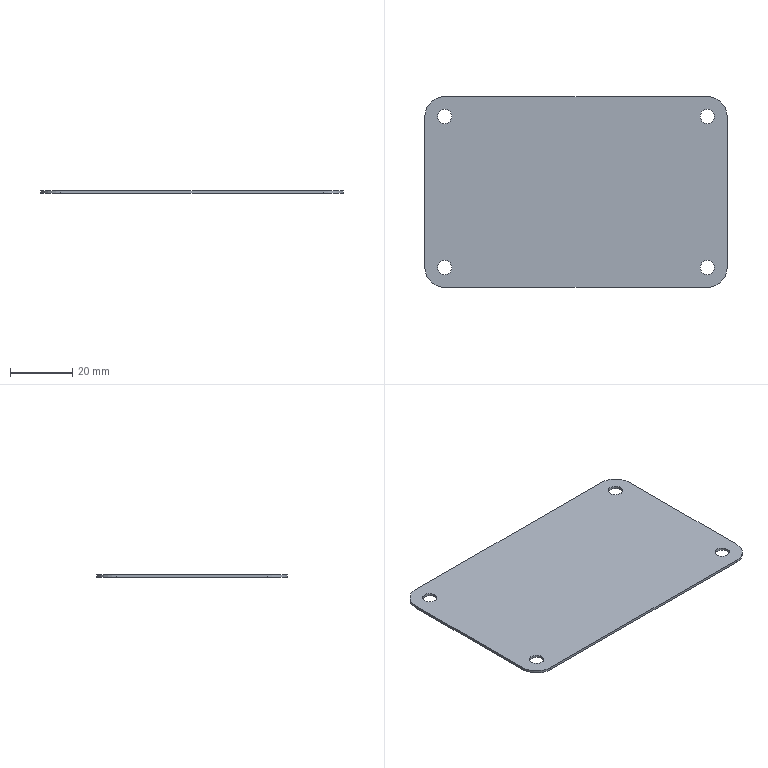Part | NX | features MG0330 trunion parts 24(steering fork) 2 | 1 solid | 14 faces | box 96.838 x 61.119 x 0.8128 mm | volume 4729 mm3 | cylinder 8 | plane 6 | commonest cylinder face diameters 4.572 x4 12.7 x4
STEP:
#1=CARTESIAN_POINT('',(44.355,-60.325,13.513));
#2=VERTEX_POINT('',#1);
#3=CARTESIAN_POINT('',(42.069,-60.325,13.513));
#4=DIRECTION('',(0.,0.,1.));
#5=DIRECTION('',(1.,0.,0.));
#6=AXIS2_PLACEMENT_3D('',#3,#4,#5);
#7=CIRCLE('',#6,2.286);
#8=EDGE_CURVE('',#2,#2,#7,.T.);
#9=ORIENTED_EDGE('',*,*,#8,.F.);
#10=EDGE_LOOP('',(#9));
#11=FACE_BOUND('',#10,.T.);
#12=CARTESIAN_POINT('',(-39.783,-108.744,13.513));
#13=VERTEX_POINT('',#12);
#14=CARTESIAN_POINT('',(-42.069,-108.744,13.513));
#15=DIRECTION('',(0.,0.,1.));
#16=DIRECTION('',(1.,0.,0.));
#17=AXIS2_PLACEMENT_3D('',#14,#15,#16);
#18=CIRCLE('',#17,2.286);
#19=EDGE_CURVE('',#13,#13,#18,.T.);
#20=ORIENTED_EDGE('',*,*,#19,.F.);
#21=EDGE_LOOP('',(#20));
#22=FACE_BOUND('',#21,.T.);
#23=CARTESIAN_POINT('',(-48.419,-60.325,13.513));
#24=VERTEX_POINT('',#23);
#25=CARTESIAN_POINT('',(-48.419,-108.744,13.513));
#26=VERTEX_POINT('',#25);
#27=CARTESIAN_POINT('',(-48.419,-53.975,13.513));
#28=DIRECTION('',(0.,-1.,0.));
#29=VECTOR('',#28,1000.);
#30=LINE('',#27,#29);
#31=EDGE_CURVE('',#24,#26,#30,.T.);
#32=ORIENTED_EDGE('',*,*,#31,.T.);
#33=CARTESIAN_POINT('',(-42.069,-115.094,13.513));
#34=VERTEX_POINT('',#33);
#35=CARTESIAN_POINT('',(-42.069,-108.744,13.513));
#36=DIRECTION('',(0.,0.,1.));
#37=DIRECTION('',(1.,0.,0.));
#38=AXIS2_PLACEMENT_3D('',#35,#36,#37);
#39=CIRCLE('',#38,6.35);
#40=EDGE_CURVE('',#26,#34,#39,.T.);
#41=ORIENTED_EDGE('',*,*,#40,.T.);
#42=CARTESIAN_POINT('',(42.069,-115.094,13.513));
#43=VERTEX_POINT('',#42);
#44=CARTESIAN_POINT('',(-48.419,-115.094,13.513));
#45=DIRECTION('',(1.,0.,0.));
#46=VECTOR('',#45,1000.);
#47=LINE('',#44,#46);
#48=EDGE_CURVE('',#34,#43,#47,.T.);
#49=ORIENTED_EDGE('',*,*,#48,.T.);
#50=CARTESIAN_POINT('',(48.419,-108.744,13.513));
#51=VERTEX_POINT('',#50);
#52=CARTESIAN_POINT('',(42.069,-108.744,13.513));
#53=DIRECTION('',(0.,0.,1.));
#54=DIRECTION('',(1.,0.,0.));
#55=AXIS2_PLACEMENT_3D('',#52,#53,#54);
#56=CIRCLE('',#55,6.35);
#57=EDGE_CURVE('',#43,#51,#56,.T.);
#58=ORIENTED_EDGE('',*,*,#57,.T.);
#59=CARTESIAN_POINT('',(48.419,-60.325,13.513));
#60=VERTEX_POINT('',#59);
#61=CARTESIAN_POINT('',(48.419,-115.094,13.513));
#62=DIRECTION('',(0.,1.,0.));
#63=VECTOR('',#62,1000.);
#64=LINE('',#61,#63);
#65=EDGE_CURVE('',#51,#60,#64,.T.);
#66=ORIENTED_EDGE('',*,*,#65,.T.);
#67=CARTESIAN_POINT('',(42.069,-53.975,13.513));
#68=VERTEX_POINT('',#67);
#69=CARTESIAN_POINT('',(42.069,-60.325,13.513));
#70=DIRECTION('',(0.,0.,1.));
#71=DIRECTION('',(1.,0.,0.));
#72=AXIS2_PLACEMENT_3D('',#69,#70,#71);
#73=CIRCLE('',#72,6.35);
#74=EDGE_CURVE('',#60,#68,#73,.T.);
#75=ORIENTED_EDGE('',*,*,#74,.T.);
#76=CARTESIAN_POINT('',(-42.069,-53.975,13.513));
#77=VERTEX_POINT('',#76);
#78=CARTESIAN_POINT('',(29.369,-53.975,13.513));
#79=DIRECTION('',(-1.,0.,0.));
#80=VECTOR('',#79,1000.);
#81=LINE('',#78,#80);
#82=EDGE_CURVE('',#68,#77,#81,.T.);
#83=ORIENTED_EDGE('',*,*,#82,.T.);
#84=CARTESIAN_POINT('',(-42.069,-60.325,13.513));
#85=DIRECTION('',(0.,0.,1.));
#86=DIRECTION('',(1.,0.,0.));
#87=AXIS2_PLACEMENT_3D('',#84,#85,#86);
#88=CIRCLE('',#87,6.35);
#89=EDGE_CURVE('',#77,#24,#88,.T.);
#90=ORIENTED_EDGE('',*,*,#89,.T.);
#91=EDGE_LOOP('',(#32,#41,#49,#58,#66,#75,#83,#90));
#92=FACE_BOUND('',#91,.T.);
#93=CARTESIAN_POINT('',(-39.783,-60.325,13.513));
#94=VERTEX_POINT('',#93);
#95=CARTESIAN_POINT('',(-42.069,-60.325,13.513));
#96=DIRECTION('',(0.,0.,1.));
#97=DIRECTION('',(1.,0.,0.));
#98=AXIS2_PLACEMENT_3D('',#95,#96,#97);
#99=CIRCLE('',#98,2.286);
#100=EDGE_CURVE('',#94,#94,#99,.T.);
#101=ORIENTED_EDGE('',*,*,#100,.F.);
#102=EDGE_LOOP('',(#101));
#103=FACE_BOUND('',#102,.T.);
#104=CARTESIAN_POINT('',(44.355,-108.744,13.513));
#105=VERTEX_POINT('',#104);
#106=CARTESIAN_POINT('',(42.069,-108.744,13.513));
#107=DIRECTION('',(0.,0.,1.));
#108=DIRECTION('',(1.,0.,0.));
#109=AXIS2_PLACEMENT_3D('',#106,#107,#108);
#110=CIRCLE('',#109,2.286);
#111=EDGE_CURVE('',#105,#105,#110,.T.);
#112=ORIENTED_EDGE('',*,*,#111,.F.);
#113=EDGE_LOOP('',(#112));
#114=FACE_BOUND('',#113,.T.);
#115=CARTESIAN_POINT('',(-48.419,-53.975,13.513));
#116=DIRECTION('',(0.,0.,1.));
#117=DIRECTION('',(1.,0.,0.));
#118=AXIS2_PLACEMENT_3D('',#115,#116,#117);
#119=PLANE('',#118);
#120=ADVANCED_FACE('',(#11,#22,#92,#103,#114),#119,.T.);
#121=CARTESIAN_POINT('',(-42.069,-115.094,12.7));
#122=VERTEX_POINT('',#121);
#123=CARTESIAN_POINT('',(42.069,-115.094,12.7));
#124=VERTEX_POINT('',#123);
#125=CARTESIAN_POINT('',(-48.419,-115.094,12.7));
#126=DIRECTION('',(1.,0.,0.));
#127=VECTOR('',#126,1000.);
#128=LINE('',#125,#127);
#129=EDGE_CURVE('',#122,#124,#128,.T.);
#130=ORIENTED_EDGE('',*,*,#129,.F.);
#131=CARTESIAN_POINT('',(-48.419,-108.744,12.7));
#132=VERTEX_POINT('',#131);
#133=CARTESIAN_POINT('',(-42.069,-108.744,12.7));
#134=DIRECTION('',(0.,0.,1.));
#135=DIRECTION('',(1.,0.,0.));
#136=AXIS2_PLACEMENT_3D('',#133,#134,#135);
#137=CIRCLE('',#136,6.35);
#138=EDGE_CURVE('',#122,#132,#137,.F.);
#139=ORIENTED_EDGE('',*,*,#138,.T.);
#140=CARTESIAN_POINT('',(-48.419,-60.325,12.7));
#141=VERTEX_POINT('',#140);
#142=CARTESIAN_POINT('',(-48.419,-53.975,12.7));
#143=DIRECTION('',(0.,-1.,0.));
#144=VECTOR('',#143,1000.);
#145=LINE('',#142,#144);
#146=EDGE_CURVE('',#141,#132,#145,.T.);
#147=ORIENTED_EDGE('',*,*,#146,.F.);
#148=CARTESIAN_POINT('',(-42.069,-53.975,12.7));
#149=VERTEX_POINT('',#148);
#150=CARTESIAN_POINT('',(-42.069,-60.325,12.7));
#151=DIRECTION('',(0.,0.,1.));
#152=DIRECTION('',(1.,0.,0.));
#153=AXIS2_PLACEMENT_3D('',#150,#151,#152);
#154=CIRCLE('',#153,6.35);
#155=EDGE_CURVE('',#141,#149,#154,.F.);
#156=ORIENTED_EDGE('',*,*,#155,.T.);
#157=CARTESIAN_POINT('',(42.069,-53.975,12.7));
#158=VERTEX_POINT('',#157);
#159=CARTESIAN_POINT('',(48.419,-53.975,12.7));
#160=DIRECTION('',(-1.,0.,0.));
#161=VECTOR('',#160,1000.);
#162=LINE('',#159,#161);
#163=EDGE_CURVE('',#158,#149,#162,.T.);
#164=ORIENTED_EDGE('',*,*,#163,.F.);
#165=CARTESIAN_POINT('',(48.419,-60.325,12.7));
#166=VERTEX_POINT('',#165);
#167=CARTESIAN_POINT('',(42.069,-60.325,12.7));
#168=DIRECTION('',(0.,0.,1.));
#169=DIRECTION('',(1.,0.,0.));
#170=AXIS2_PLACEMENT_3D('',#167,#168,#169);
#171=CIRCLE('',#170,6.35);
#172=EDGE_CURVE('',#158,#166,#171,.F.);
#173=ORIENTED_EDGE('',*,*,#172,.T.);
#174=CARTESIAN_POINT('',(48.419,-108.744,12.7));
#175=VERTEX_POINT('',#174);
#176=CARTESIAN_POINT('',(48.419,-115.094,12.7));
#177=DIRECTION('',(0.,1.,0.));
#178=VECTOR('',#177,1000.);
#179=LINE('',#176,#178);
#180=EDGE_CURVE('',#175,#166,#179,.T.);
#181=ORIENTED_EDGE('',*,*,#180,.F.);
#182=CARTESIAN_POINT('',(42.069,-108.744,12.7));
#183=DIRECTION('',(0.,0.,1.));
#184=DIRECTION('',(1.,0.,0.));
#185=AXIS2_PLACEMENT_3D('',#182,#183,#184);
#186=CIRCLE('',#185,6.35);
#187=EDGE_CURVE('',#175,#124,#186,.F.);
#188=ORIENTED_EDGE('',*,*,#187,.T.);
#189=EDGE_LOOP('',(#130,#139,#147,#156,#164,#173,#181,#188));
#190=FACE_BOUND('',#189,.T.);
#191=CARTESIAN_POINT('',(-39.783,-108.744,12.7));
#192=VERTEX_POINT('',#191);
#193=CARTESIAN_POINT('',(-42.069,-108.744,12.7));
#194=DIRECTION('',(0.,0.,1.));
#195=DIRECTION('',(1.,0.,0.));
#196=AXIS2_PLACEMENT_3D('',#193,#194,#195);
#197=CIRCLE('',#196,2.286);
#198=EDGE_CURVE('',#192,#192,#197,.T.);
#199=ORIENTED_EDGE('',*,*,#198,.T.);
#200=EDGE_LOOP('',(#199));
#201=FACE_BOUND('',#200,.T.);
#202=CARTESIAN_POINT('',(-39.783,-60.325,12.7));
#203=VERTEX_POINT('',#202);
#204=CARTESIAN_POINT('',(-42.069,-60.325,12.7));
#205=DIRECTION('',(0.,0.,1.));
#206=DIRECTION('',(1.,0.,0.));
#207=AXIS2_PLACEMENT_3D('',#204,#205,#206);
#208=CIRCLE('',#207,2.286);
#209=EDGE_CURVE('',#203,#203,#208,.T.);
#210=ORIENTED_EDGE('',*,*,#209,.T.);
#211=EDGE_LOOP('',(#210));
#212=FACE_BOUND('',#211,.T.);
#213=CARTESIAN_POINT('',(44.355,-60.325,12.7));
#214=VERTEX_POINT('',#213);
#215=CARTESIAN_POINT('',(42.069,-60.325,12.7));
#216=DIRECTION('',(0.,0.,1.));
#217=DIRECTION('',(1.,0.,0.));
#218=AXIS2_PLACEMENT_3D('',#215,#216,#217);
#219=CIRCLE('',#218,2.286);
#220=EDGE_CURVE('',#214,#214,#219,.T.);
#221=ORIENTED_EDGE('',*,*,#220,.T.);
#222=EDGE_LOOP('',(#221));
#223=FACE_BOUND('',#222,.T.);
#224=CARTESIAN_POINT('',(44.355,-108.744,12.7));
#225=VERTEX_POINT('',#224);
#226=CARTESIAN_POINT('',(42.069,-108.744,12.7));
#227=DIRECTION('',(0.,0.,1.));
#228=DIRECTION('',(1.,0.,0.));
#229=AXIS2_PLACEMENT_3D('',#226,#227,#228);
#230=CIRCLE('',#229,2.286);
#231=EDGE_CURVE('',#225,#225,#230,.T.);
#232=ORIENTED_EDGE('',*,*,#231,.T.);
#233=EDGE_LOOP('',(#232));
#234=FACE_BOUND('',#233,.T.);
#235=CARTESIAN_POINT('',(-48.419,-53.975,12.7));
#236=DIRECTION('',(0.,0.,1.));
#237=DIRECTION('',(1.,0.,0.));
#238=AXIS2_PLACEMENT_3D('',#235,#236,#237);
#239=PLANE('',#238);
#240=ADVANCED_FACE('',(#190,#201,#212,#223,#234),#239,.F.);
#241=ORIENTED_EDGE('',*,*,#146,.T.);
#242=CARTESIAN_POINT('',(-48.419,-108.744,13.513));
#243=DIRECTION('',(0.,0.,-1.));
#244=VECTOR('',#243,1000.);
#245=LINE('',#242,#244);
#246=EDGE_CURVE('',#132,#26,#245,.F.);
#247=ORIENTED_EDGE('',*,*,#246,.T.);
#248=ORIENTED_EDGE('',*,*,#31,.F.);
#249=CARTESIAN_POINT('',(-48.419,-60.325,13.513));
#250=DIRECTION('',(0.,0.,-1.));
#251=VECTOR('',#250,1000.);
#252=LINE('',#249,#251);
#253=EDGE_CURVE('',#24,#141,#252,.T.);
#254=ORIENTED_EDGE('',*,*,#253,.T.);
#255=EDGE_LOOP('',(#241,#247,#248,#254));
#256=FACE_BOUND('',#255,.T.);
#257=CARTESIAN_POINT('',(-48.419,-53.975,13.513));
#258=DIRECTION('',(1.,0.,0.));
#259=DIRECTION('',(0.,1.,0.));
#260=AXIS2_PLACEMENT_3D('',#257,#258,#259);
#261=PLANE('',#260);
#262=ADVANCED_FACE('',(#256),#261,.F.);
#263=ORIENTED_EDGE('',*,*,#48,.F.);
#264=CARTESIAN_POINT('',(-42.069,-115.094,13.513));
#265=DIRECTION('',(0.,0.,-1.));
#266=VECTOR('',#265,1000.);
#267=LINE('',#264,#266);
#268=EDGE_CURVE('',#34,#122,#267,.T.);
#269=ORIENTED_EDGE('',*,*,#268,.T.);
#270=ORIENTED_EDGE('',*,*,#129,.T.);
#271=CARTESIAN_POINT('',(42.069,-115.094,13.513));
#272=DIRECTION('',(0.,0.,-1.));
#273=VECTOR('',#272,1000.);
#274=LINE('',#271,#273);
#275=EDGE_CURVE('',#124,#43,#274,.F.);
#276=ORIENTED_EDGE('',*,*,#275,.T.);
#277=EDGE_LOOP('',(#263,#269,#270,#276));
#278=FACE_BOUND('',#277,.T.);
#279=CARTESIAN_POINT('',(-48.419,-115.094,13.513));
#280=DIRECTION('',(0.,1.,0.));
#281=DIRECTION('',(0.,0.,1.));
#282=AXIS2_PLACEMENT_3D('',#279,#280,#281);
#283=PLANE('',#282);
#284=ADVANCED_FACE('',(#278),#283,.F.);
#285=ORIENTED_EDGE('',*,*,#65,.F.);
#286=CARTESIAN_POINT('',(48.419,-108.744,13.513));
#287=DIRECTION('',(0.,0.,-1.));
#288=VECTOR('',#287,1000.);
#289=LINE('',#286,#288);
#290=EDGE_CURVE('',#51,#175,#289,.T.);
#291=ORIENTED_EDGE('',*,*,#290,.T.);
#292=ORIENTED_EDGE('',*,*,#180,.T.);
#293=CARTESIAN_POINT('',(48.419,-60.325,13.513));
#294=DIRECTION('',(0.,0.,-1.));
#295=VECTOR('',#294,1000.);
#296=LINE('',#293,#295);
#297=EDGE_CURVE('',#166,#60,#296,.F.);
#298=ORIENTED_EDGE('',*,*,#297,.T.);
#299=EDGE_LOOP('',(#285,#291,#292,#298));
#300=FACE_BOUND('',#299,.T.);
#301=CARTESIAN_POINT('',(48.419,-115.094,13.513));
#302=DIRECTION('',(-1.,0.,0.));
#303=DIRECTION('',(0.,-1.,0.));
#304=AXIS2_PLACEMENT_3D('',#301,#302,#303);
#305=PLANE('',#304);
#306=ADVANCED_FACE('',(#300),#305,.F.);
#307=ORIENTED_EDGE('',*,*,#163,.T.);
#308=CARTESIAN_POINT('',(-42.069,-53.975,13.513));
#309=DIRECTION('',(0.,0.,-1.));
#310=VECTOR('',#309,1000.);
#311=LINE('',#308,#310);
#312=EDGE_CURVE('',#149,#77,#311,.F.);
#313=ORIENTED_EDGE('',*,*,#312,.T.);
#314=ORIENTED_EDGE('',*,*,#82,.F.);
#315=CARTESIAN_POINT('',(42.069,-53.975,13.513));
#316=DIRECTION('',(0.,0.,-1.));
#317=VECTOR('',#316,1000.);
#318=LINE('',#315,#317);
#319=EDGE_CURVE('',#68,#158,#318,.T.);
#320=ORIENTED_EDGE('',*,*,#319,.T.);
#321=EDGE_LOOP('',(#307,#313,#314,#320));
#322=FACE_BOUND('',#321,.T.);
#323=CARTESIAN_POINT('',(48.419,-53.975,13.513));
#324=DIRECTION('',(0.,-1.,0.));
#325=DIRECTION('',(1.,0.,0.));
#326=AXIS2_PLACEMENT_3D('',#323,#324,#325);
#327=PLANE('',#326);
#328=ADVANCED_FACE('',(#322),#327,.F.);
#329=ORIENTED_EDGE('',*,*,#19,.T.);
#330=EDGE_LOOP('',(#329));
#331=FACE_BOUND('',#330,.T.);
#332=ORIENTED_EDGE('',*,*,#198,.F.);
#333=EDGE_LOOP('',(#332));
#334=FACE_BOUND('',#333,.T.);
#335=CARTESIAN_POINT('',(-42.069,-108.744,13.513));
#336=DIRECTION('',(0.,0.,-1.));
#337=DIRECTION('',(-1.,0.,0.));
#338=AXIS2_PLACEMENT_3D('',#335,#336,#337);
#339=CYLINDRICAL_SURFACE('',#338,2.286);
#340=ADVANCED_FACE('',(#331,#334),#339,.F.);
#341=ORIENTED_EDGE('',*,*,#100,.T.);
#342=EDGE_LOOP('',(#341));
#343=FACE_BOUND('',#342,.T.);
#344=ORIENTED_EDGE('',*,*,#209,.F.);
#345=EDGE_LOOP('',(#344));
#346=FACE_BOUND('',#345,.T.);
#347=CARTESIAN_POINT('',(-42.069,-60.325,13.513));
#348=DIRECTION('',(0.,0.,-1.));
#349=DIRECTION('',(-1.,0.,0.));
#350=AXIS2_PLACEMENT_3D('',#347,#348,#349);
#351=CYLINDRICAL_SURFACE('',#350,2.286);
#352=ADVANCED_FACE('',(#343,#346),#351,.F.);
#353=ORIENTED_EDGE('',*,*,#8,.T.);
#354=EDGE_LOOP('',(#353));
#355=FACE_BOUND('',#354,.T.);
#356=ORIENTED_EDGE('',*,*,#220,.F.);
#357=EDGE_LOOP('',(#356));
#358=FACE_BOUND('',#357,.T.);
#359=CARTESIAN_POINT('',(42.069,-60.325,13.513));
#360=DIRECTION('',(0.,0.,-1.));
#361=DIRECTION('',(-1.,0.,0.));
#362=AXIS2_PLACEMENT_3D('',#359,#360,#361);
#363=CYLINDRICAL_SURFACE('',#362,2.286);
#364=ADVANCED_FACE('',(#355,#358),#363,.F.);
#365=ORIENTED_EDGE('',*,*,#111,.T.);
#366=EDGE_LOOP('',(#365));
#367=FACE_BOUND('',#366,.T.);
#368=ORIENTED_EDGE('',*,*,#231,.F.);
#369=EDGE_LOOP('',(#368));
#370=FACE_BOUND('',#369,.T.);
#371=CARTESIAN_POINT('',(42.069,-108.744,13.513));
#372=DIRECTION('',(0.,0.,-1.));
#373=DIRECTION('',(-1.,0.,0.));
#374=AXIS2_PLACEMENT_3D('',#371,#372,#373);
#375=CYLINDRICAL_SURFACE('',#374,2.286);
#376=ADVANCED_FACE('',(#367,#370),#375,.F.);
#377=ORIENTED_EDGE('',*,*,#40,.F.);
#378=ORIENTED_EDGE('',*,*,#246,.F.);
#379=ORIENTED_EDGE('',*,*,#138,.F.);
#380=ORIENTED_EDGE('',*,*,#268,.F.);
#381=EDGE_LOOP('',(#377,#378,#379,#380));
#382=FACE_BOUND('',#381,.T.);
#383=CARTESIAN_POINT('',(-42.069,-108.744,13.513));
#384=DIRECTION('',(0.,0.,-1.));
#385=DIRECTION('',(-1.,0.,0.));
#386=AXIS2_PLACEMENT_3D('',#383,#384,#385);
#387=CYLINDRICAL_SURFACE('',#386,6.35);
#388=ADVANCED_FACE('',(#382),#387,.T.);
#389=ORIENTED_EDGE('',*,*,#89,.F.);
#390=ORIENTED_EDGE('',*,*,#312,.F.);
#391=ORIENTED_EDGE('',*,*,#155,.F.);
#392=ORIENTED_EDGE('',*,*,#253,.F.);
#393=EDGE_LOOP('',(#389,#390,#391,#392));
#394=FACE_BOUND('',#393,.T.);
#395=CARTESIAN_POINT('',(-42.069,-60.325,13.513));
#396=DIRECTION('',(0.,0.,-1.));
#397=DIRECTION('',(-1.,0.,0.));
#398=AXIS2_PLACEMENT_3D('',#395,#396,#397);
#399=CYLINDRICAL_SURFACE('',#398,6.35);
#400=ADVANCED_FACE('',(#394),#399,.T.);
#401=ORIENTED_EDGE('',*,*,#57,.F.);
#402=ORIENTED_EDGE('',*,*,#275,.F.);
#403=ORIENTED_EDGE('',*,*,#187,.F.);
#404=ORIENTED_EDGE('',*,*,#290,.F.);
#405=EDGE_LOOP('',(#401,#402,#403,#404));
#406=FACE_BOUND('',#405,.T.);
#407=CARTESIAN_POINT('',(42.069,-108.744,13.513));
#408=DIRECTION('',(0.,0.,-1.));
#409=DIRECTION('',(-1.,0.,0.));
#410=AXIS2_PLACEMENT_3D('',#407,#408,#409);
#411=CYLINDRICAL_SURFACE('',#410,6.35);
#412=ADVANCED_FACE('',(#406),#411,.T.);
#413=ORIENTED_EDGE('',*,*,#74,.F.);
#414=ORIENTED_EDGE('',*,*,#297,.F.);
#415=ORIENTED_EDGE('',*,*,#172,.F.);
#416=ORIENTED_EDGE('',*,*,#319,.F.);
#417=EDGE_LOOP('',(#413,#414,#415,#416));
#418=FACE_BOUND('',#417,.T.);
#419=CARTESIAN_POINT('',(42.069,-60.325,13.513));
#420=DIRECTION('',(0.,0.,-1.));
#421=DIRECTION('',(-1.,0.,0.));
#422=AXIS2_PLACEMENT_3D('',#419,#420,#421);
#423=CYLINDRICAL_SURFACE('',#422,6.35);
#424=ADVANCED_FACE('',(#418),#423,.T.);
#425=CLOSED_SHELL('',(#120,#240,#262,#284,#306,#328,#340,#352,#364,#376,#388,#400,#412,#424));
#426=MANIFOLD_SOLID_BREP('',#425);
#427=(LENGTH_UNIT()NAMED_UNIT(*)SI_UNIT(.MILLI.,.METRE.));
#428=UNCERTAINTY_MEASURE_WITH_UNIT(LENGTH_MEASURE(0.00001),#427,'','');
#429=(NAMED_UNIT(*)PLANE_ANGLE_UNIT()SI_UNIT($,.RADIAN.));
#430=(NAMED_UNIT(*)SI_UNIT($,.STERADIAN.)SOLID_ANGLE_UNIT());
#431=(GEOMETRIC_REPRESENTATION_CONTEXT(3)GLOBAL_UNCERTAINTY_ASSIGNED_CONTEXT((#428))GLOBAL_UNIT_ASSIGNED_CONTEXT((#427,#429,#430))REPRESENTATION_CONTEXT('',''));
#432=ADVANCED_BREP_SHAPE_REPRESENTATION('',(#426),#431);